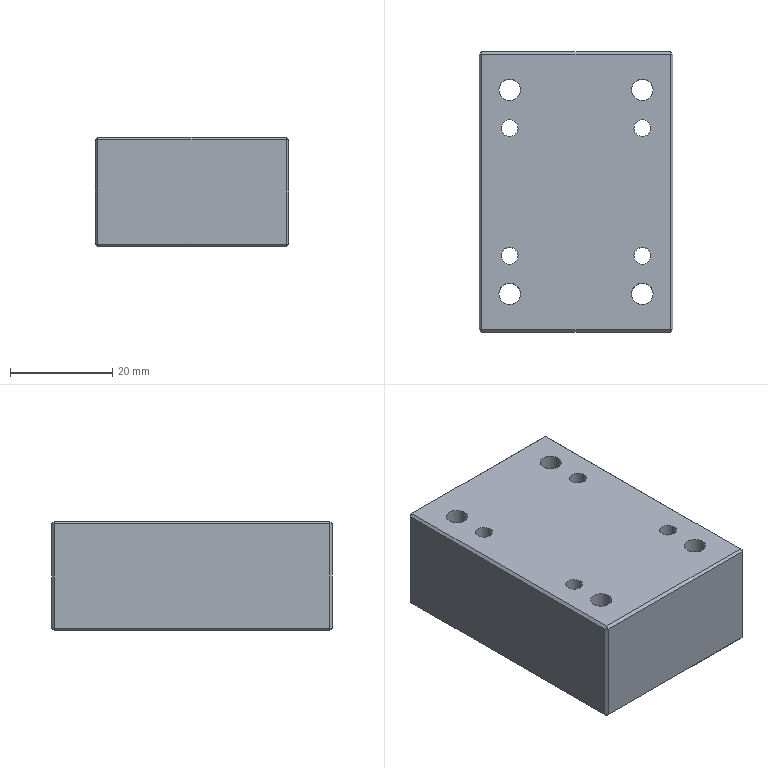Part | NX | 1 solid | 34 faces | box 38 x 55 x 21.5 mm | volume 42951 mm3 | plane 26 | cylinder 8 | commonest cylinder face diameters 3.3 x4 4.2 x4
STEP:
#1=CARTESIAN_POINT('',(-19.,-27.,0.5));
#2=VERTEX_POINT('',#1);
#3=CARTESIAN_POINT('',(-19.,-27.,21.));
#4=VERTEX_POINT('',#3);
#5=CARTESIAN_POINT('',(-19.,-27.,21.5));
#6=DIRECTION('',(0.,0.,1.));
#7=VECTOR('',#6,1000.);
#8=LINE('',#5,#7);
#9=EDGE_CURVE('',#2,#4,#8,.T.);
#10=ORIENTED_EDGE('',*,*,#9,.T.);
#11=CARTESIAN_POINT('',(-19.,27.,21.));
#12=VERTEX_POINT('',#11);
#13=CARTESIAN_POINT('',(-19.,27.5,21.));
#14=DIRECTION('',(0.,1.,0.));
#15=VECTOR('',#14,1000.);
#16=LINE('',#13,#15);
#17=EDGE_CURVE('',#4,#12,#16,.T.);
#18=ORIENTED_EDGE('',*,*,#17,.T.);
#19=CARTESIAN_POINT('',(-19.,27.,0.5));
#20=VERTEX_POINT('',#19);
#21=CARTESIAN_POINT('',(-19.,27.,21.5));
#22=DIRECTION('',(0.,0.,-1.));
#23=VECTOR('',#22,1000.);
#24=LINE('',#21,#23);
#25=EDGE_CURVE('',#12,#20,#24,.T.);
#26=ORIENTED_EDGE('',*,*,#25,.T.);
#27=CARTESIAN_POINT('',(-19.,-27.5,0.5));
#28=DIRECTION('',(0.,-1.,0.));
#29=VECTOR('',#28,1000.);
#30=LINE('',#27,#29);
#31=EDGE_CURVE('',#20,#2,#30,.T.);
#32=ORIENTED_EDGE('',*,*,#31,.T.);
#33=EDGE_LOOP('',(#10,#18,#26,#32));
#34=FACE_BOUND('',#33,.T.);
#35=CARTESIAN_POINT('',(-19.,27.5,21.5));
#36=DIRECTION('',(1.,0.,0.));
#37=DIRECTION('',(0.,1.,0.));
#38=AXIS2_PLACEMENT_3D('',#35,#36,#37);
#39=PLANE('',#38);
#40=ADVANCED_FACE('',(#34),#39,.F.);
#41=CARTESIAN_POINT('',(18.5,-27.5,21.));
#42=VERTEX_POINT('',#41);
#43=CARTESIAN_POINT('',(-18.5,-27.5,21.));
#44=VERTEX_POINT('',#43);
#45=CARTESIAN_POINT('',(19.,-27.5,21.));
#46=DIRECTION('',(-1.,0.,0.));
#47=VECTOR('',#46,1000.);
#48=LINE('',#45,#47);
#49=EDGE_CURVE('',#42,#44,#48,.T.);
#50=ORIENTED_EDGE('',*,*,#49,.T.);
#51=CARTESIAN_POINT('',(-18.5,-27.5,0.5));
#52=VERTEX_POINT('',#51);
#53=CARTESIAN_POINT('',(-18.5,-27.5,21.5));
#54=DIRECTION('',(0.,0.,-1.));
#55=VECTOR('',#54,1000.);
#56=LINE('',#53,#55);
#57=EDGE_CURVE('',#44,#52,#56,.T.);
#58=ORIENTED_EDGE('',*,*,#57,.T.);
#59=CARTESIAN_POINT('',(18.5,-27.5,0.5));
#60=VERTEX_POINT('',#59);
#61=CARTESIAN_POINT('',(19.,-27.5,0.5));
#62=DIRECTION('',(1.,0.,0.));
#63=VECTOR('',#62,1000.);
#64=LINE('',#61,#63);
#65=EDGE_CURVE('',#52,#60,#64,.T.);
#66=ORIENTED_EDGE('',*,*,#65,.T.);
#67=CARTESIAN_POINT('',(18.5,-27.5,21.5));
#68=DIRECTION('',(0.,0.,1.));
#69=VECTOR('',#68,1000.);
#70=LINE('',#67,#69);
#71=EDGE_CURVE('',#60,#42,#70,.T.);
#72=ORIENTED_EDGE('',*,*,#71,.T.);
#73=EDGE_LOOP('',(#50,#58,#66,#72));
#74=FACE_BOUND('',#73,.T.);
#75=CARTESIAN_POINT('',(19.,-27.5,21.5));
#76=DIRECTION('',(0.,1.,0.));
#77=DIRECTION('',(-1.,0.,0.));
#78=AXIS2_PLACEMENT_3D('',#75,#76,#77);
#79=PLANE('',#78);
#80=ADVANCED_FACE('',(#74),#79,.F.);
#81=CARTESIAN_POINT('',(19.,-27.,0.5));
#82=VERTEX_POINT('',#81);
#83=CARTESIAN_POINT('',(19.,27.,0.5));
#84=VERTEX_POINT('',#83);
#85=CARTESIAN_POINT('',(19.,27.5,0.5));
#86=DIRECTION('',(0.,1.,0.));
#87=VECTOR('',#86,1000.);
#88=LINE('',#85,#87);
#89=EDGE_CURVE('',#82,#84,#88,.T.);
#90=ORIENTED_EDGE('',*,*,#89,.T.);
#91=CARTESIAN_POINT('',(19.,27.,21.));
#92=VERTEX_POINT('',#91);
#93=CARTESIAN_POINT('',(19.,27.,21.5));
#94=DIRECTION('',(0.,0.,1.));
#95=VECTOR('',#94,1000.);
#96=LINE('',#93,#95);
#97=EDGE_CURVE('',#84,#92,#96,.T.);
#98=ORIENTED_EDGE('',*,*,#97,.T.);
#99=CARTESIAN_POINT('',(19.,-27.,21.));
#100=VERTEX_POINT('',#99);
#101=CARTESIAN_POINT('',(19.,27.5,21.));
#102=DIRECTION('',(0.,-1.,0.));
#103=VECTOR('',#102,1000.);
#104=LINE('',#101,#103);
#105=EDGE_CURVE('',#92,#100,#104,.T.);
#106=ORIENTED_EDGE('',*,*,#105,.T.);
#107=CARTESIAN_POINT('',(19.,-27.,21.5));
#108=DIRECTION('',(0.,0.,-1.));
#109=VECTOR('',#108,1000.);
#110=LINE('',#107,#109);
#111=EDGE_CURVE('',#100,#82,#110,.T.);
#112=ORIENTED_EDGE('',*,*,#111,.T.);
#113=EDGE_LOOP('',(#90,#98,#106,#112));
#114=FACE_BOUND('',#113,.T.);
#115=CARTESIAN_POINT('',(19.,27.5,21.5));
#116=DIRECTION('',(-1.,0.,0.));
#117=DIRECTION('',(0.,-1.,0.));
#118=AXIS2_PLACEMENT_3D('',#115,#116,#117);
#119=PLANE('',#118);
#120=ADVANCED_FACE('',(#114),#119,.F.);
#121=CARTESIAN_POINT('',(-18.5,27.5,21.));
#122=VERTEX_POINT('',#121);
#123=CARTESIAN_POINT('',(18.5,27.5,21.));
#124=VERTEX_POINT('',#123);
#125=CARTESIAN_POINT('',(19.,27.5,21.));
#126=DIRECTION('',(1.,0.,0.));
#127=VECTOR('',#126,1000.);
#128=LINE('',#125,#127);
#129=EDGE_CURVE('',#122,#124,#128,.T.);
#130=ORIENTED_EDGE('',*,*,#129,.T.);
#131=CARTESIAN_POINT('',(18.5,27.5,0.5));
#132=VERTEX_POINT('',#131);
#133=CARTESIAN_POINT('',(18.5,27.5,21.5));
#134=DIRECTION('',(0.,0.,-1.));
#135=VECTOR('',#134,1000.);
#136=LINE('',#133,#135);
#137=EDGE_CURVE('',#124,#132,#136,.T.);
#138=ORIENTED_EDGE('',*,*,#137,.T.);
#139=CARTESIAN_POINT('',(-18.5,27.5,0.5));
#140=VERTEX_POINT('',#139);
#141=CARTESIAN_POINT('',(-19.,27.5,0.5));
#142=DIRECTION('',(-1.,0.,0.));
#143=VECTOR('',#142,1000.);
#144=LINE('',#141,#143);
#145=EDGE_CURVE('',#132,#140,#144,.T.);
#146=ORIENTED_EDGE('',*,*,#145,.T.);
#147=CARTESIAN_POINT('',(-18.5,27.5,21.5));
#148=DIRECTION('',(0.,0.,1.));
#149=VECTOR('',#148,1000.);
#150=LINE('',#147,#149);
#151=EDGE_CURVE('',#140,#122,#150,.T.);
#152=ORIENTED_EDGE('',*,*,#151,.T.);
#153=EDGE_LOOP('',(#130,#138,#146,#152));
#154=FACE_BOUND('',#153,.T.);
#155=CARTESIAN_POINT('',(19.,27.5,21.5));
#156=DIRECTION('',(0.,-1.,0.));
#157=DIRECTION('',(1.,0.,0.));
#158=AXIS2_PLACEMENT_3D('',#155,#156,#157);
#159=PLANE('',#158);
#160=ADVANCED_FACE('',(#154),#159,.F.);
#161=CARTESIAN_POINT('',(18.5,-27.,21.5));
#162=VERTEX_POINT('',#161);
#163=CARTESIAN_POINT('',(18.5,27.,21.5));
#164=VERTEX_POINT('',#163);
#165=CARTESIAN_POINT('',(18.5,0.,21.5));
#166=DIRECTION('',(0.,1.,0.));
#167=VECTOR('',#166,1000.);
#168=LINE('',#165,#167);
#169=EDGE_CURVE('',#162,#164,#168,.T.);
#170=ORIENTED_EDGE('',*,*,#169,.T.);
#171=CARTESIAN_POINT('',(-18.5,27.,21.5));
#172=VERTEX_POINT('',#171);
#173=CARTESIAN_POINT('',(0.,27.,21.5));
#174=DIRECTION('',(-1.,0.,0.));
#175=VECTOR('',#174,1000.);
#176=LINE('',#173,#175);
#177=EDGE_CURVE('',#164,#172,#176,.T.);
#178=ORIENTED_EDGE('',*,*,#177,.T.);
#179=CARTESIAN_POINT('',(-18.5,-27.,21.5));
#180=VERTEX_POINT('',#179);
#181=CARTESIAN_POINT('',(-18.5,0.,21.5));
#182=DIRECTION('',(0.,-1.,0.));
#183=VECTOR('',#182,1000.);
#184=LINE('',#181,#183);
#185=EDGE_CURVE('',#172,#180,#184,.T.);
#186=ORIENTED_EDGE('',*,*,#185,.T.);
#187=CARTESIAN_POINT('',(0.,-27.,21.5));
#188=DIRECTION('',(1.,0.,0.));
#189=VECTOR('',#188,1000.);
#190=LINE('',#187,#189);
#191=EDGE_CURVE('',#180,#162,#190,.T.);
#192=ORIENTED_EDGE('',*,*,#191,.T.);
#193=EDGE_LOOP('',(#170,#178,#186,#192));
#194=FACE_BOUND('',#193,.T.);
#195=CARTESIAN_POINT('',(11.35,12.5,21.5));
#196=VERTEX_POINT('',#195);
#197=CARTESIAN_POINT('',(13.,12.5,21.5));
#198=DIRECTION('',(0.,0.,-1.));
#199=DIRECTION('',(-1.,0.,0.));
#200=AXIS2_PLACEMENT_3D('',#197,#198,#199);
#201=CIRCLE('',#200,1.65);
#202=EDGE_CURVE('',#196,#196,#201,.T.);
#203=ORIENTED_EDGE('',*,*,#202,.T.);
#204=EDGE_LOOP('',(#203));
#205=FACE_BOUND('',#204,.T.);
#206=CARTESIAN_POINT('',(-14.65,12.5,21.5));
#207=VERTEX_POINT('',#206);
#208=CARTESIAN_POINT('',(-13.,12.5,21.5));
#209=DIRECTION('',(0.,0.,-1.));
#210=DIRECTION('',(-1.,0.,0.));
#211=AXIS2_PLACEMENT_3D('',#208,#209,#210);
#212=CIRCLE('',#211,1.65);
#213=EDGE_CURVE('',#207,#207,#212,.T.);
#214=ORIENTED_EDGE('',*,*,#213,.T.);
#215=EDGE_LOOP('',(#214));
#216=FACE_BOUND('',#215,.T.);
#217=CARTESIAN_POINT('',(-14.65,-12.5,21.5));
#218=VERTEX_POINT('',#217);
#219=CARTESIAN_POINT('',(-13.,-12.5,21.5));
#220=DIRECTION('',(0.,0.,-1.));
#221=DIRECTION('',(-1.,0.,0.));
#222=AXIS2_PLACEMENT_3D('',#219,#220,#221);
#223=CIRCLE('',#222,1.65);
#224=EDGE_CURVE('',#218,#218,#223,.T.);
#225=ORIENTED_EDGE('',*,*,#224,.T.);
#226=EDGE_LOOP('',(#225));
#227=FACE_BOUND('',#226,.T.);
#228=CARTESIAN_POINT('',(11.35,-12.5,21.5));
#229=VERTEX_POINT('',#228);
#230=CARTESIAN_POINT('',(13.,-12.5,21.5));
#231=DIRECTION('',(0.,0.,-1.));
#232=DIRECTION('',(-1.,0.,0.));
#233=AXIS2_PLACEMENT_3D('',#230,#231,#232);
#234=CIRCLE('',#233,1.65);
#235=EDGE_CURVE('',#229,#229,#234,.T.);
#236=ORIENTED_EDGE('',*,*,#235,.T.);
#237=EDGE_LOOP('',(#236));
#238=FACE_BOUND('',#237,.T.);
#239=CARTESIAN_POINT('',(10.9,20.,21.5));
#240=VERTEX_POINT('',#239);
#241=CARTESIAN_POINT('',(13.,20.,21.5));
#242=DIRECTION('',(0.,0.,-1.));
#243=DIRECTION('',(-1.,0.,0.));
#244=AXIS2_PLACEMENT_3D('',#241,#242,#243);
#245=CIRCLE('',#244,2.1);
#246=EDGE_CURVE('',#240,#240,#245,.T.);
#247=ORIENTED_EDGE('',*,*,#246,.T.);
#248=EDGE_LOOP('',(#247));
#249=FACE_BOUND('',#248,.T.);
#250=CARTESIAN_POINT('',(10.9,-20.,21.5));
#251=VERTEX_POINT('',#250);
#252=CARTESIAN_POINT('',(13.,-20.,21.5));
#253=DIRECTION('',(0.,0.,-1.));
#254=DIRECTION('',(-1.,0.,0.));
#255=AXIS2_PLACEMENT_3D('',#252,#253,#254);
#256=CIRCLE('',#255,2.1);
#257=EDGE_CURVE('',#251,#251,#256,.T.);
#258=ORIENTED_EDGE('',*,*,#257,.T.);
#259=EDGE_LOOP('',(#258));
#260=FACE_BOUND('',#259,.T.);
#261=CARTESIAN_POINT('',(-15.1,-20.,21.5));
#262=VERTEX_POINT('',#261);
#263=CARTESIAN_POINT('',(-13.,-20.,21.5));
#264=DIRECTION('',(0.,0.,-1.));
#265=DIRECTION('',(-1.,0.,0.));
#266=AXIS2_PLACEMENT_3D('',#263,#264,#265);
#267=CIRCLE('',#266,2.1);
#268=EDGE_CURVE('',#262,#262,#267,.T.);
#269=ORIENTED_EDGE('',*,*,#268,.T.);
#270=EDGE_LOOP('',(#269));
#271=FACE_BOUND('',#270,.T.);
#272=CARTESIAN_POINT('',(-15.1,20.,21.5));
#273=VERTEX_POINT('',#272);
#274=CARTESIAN_POINT('',(-13.,20.,21.5));
#275=DIRECTION('',(0.,0.,-1.));
#276=DIRECTION('',(-1.,0.,0.));
#277=AXIS2_PLACEMENT_3D('',#274,#275,#276);
#278=CIRCLE('',#277,2.1);
#279=EDGE_CURVE('',#273,#273,#278,.T.);
#280=ORIENTED_EDGE('',*,*,#279,.T.);
#281=EDGE_LOOP('',(#280));
#282=FACE_BOUND('',#281,.T.);
#283=CARTESIAN_POINT('',(0.,0.,21.5));
#284=DIRECTION('',(0.,0.,-1.));
#285=DIRECTION('',(-1.,0.,0.));
#286=AXIS2_PLACEMENT_3D('',#283,#284,#285);
#287=PLANE('',#286);
#288=ADVANCED_FACE('',(#194,#205,#216,#227,#238,#249,#260,#271,#282),#287,.F.);
#289=CARTESIAN_POINT('',(-18.5,-27.,0.));
#290=VERTEX_POINT('',#289);
#291=CARTESIAN_POINT('',(-18.5,27.,0.));
#292=VERTEX_POINT('',#291);
#293=CARTESIAN_POINT('',(-18.5,27.5,0.));
#294=DIRECTION('',(0.,1.,0.));
#295=VECTOR('',#294,1000.);
#296=LINE('',#293,#295);
#297=EDGE_CURVE('',#290,#292,#296,.T.);
#298=ORIENTED_EDGE('',*,*,#297,.T.);
#299=CARTESIAN_POINT('',(18.5,27.,0.));
#300=VERTEX_POINT('',#299);
#301=CARTESIAN_POINT('',(19.,27.,0.));
#302=DIRECTION('',(1.,0.,0.));
#303=VECTOR('',#302,1000.);
#304=LINE('',#301,#303);
#305=EDGE_CURVE('',#292,#300,#304,.T.);
#306=ORIENTED_EDGE('',*,*,#305,.T.);
#307=CARTESIAN_POINT('',(18.5,-27.,0.));
#308=VERTEX_POINT('',#307);
#309=CARTESIAN_POINT('',(18.5,-27.5,0.));
#310=DIRECTION('',(0.,-1.,0.));
#311=VECTOR('',#310,1000.);
#312=LINE('',#309,#311);
#313=EDGE_CURVE('',#300,#308,#312,.T.);
#314=ORIENTED_EDGE('',*,*,#313,.T.);
#315=CARTESIAN_POINT('',(-19.,-27.,0.));
#316=DIRECTION('',(-1.,0.,0.));
#317=VECTOR('',#316,1000.);
#318=LINE('',#315,#317);
#319=EDGE_CURVE('',#308,#290,#318,.T.);
#320=ORIENTED_EDGE('',*,*,#319,.T.);
#321=EDGE_LOOP('',(#298,#306,#314,#320));
#322=FACE_BOUND('',#321,.T.);
#323=CARTESIAN_POINT('',(11.35,12.5,0.));
#324=VERTEX_POINT('',#323);
#325=CARTESIAN_POINT('',(13.,12.5,0.));
#326=DIRECTION('',(0.,0.,-1.));
#327=DIRECTION('',(-1.,0.,0.));
#328=AXIS2_PLACEMENT_3D('',#325,#326,#327);
#329=CIRCLE('',#328,1.65);
#330=EDGE_CURVE('',#324,#324,#329,.T.);
#331=ORIENTED_EDGE('',*,*,#330,.F.);
#332=EDGE_LOOP('',(#331));
#333=FACE_BOUND('',#332,.T.);
#334=CARTESIAN_POINT('',(-14.65,12.5,0.));
#335=VERTEX_POINT('',#334);
#336=CARTESIAN_POINT('',(-13.,12.5,0.));
#337=DIRECTION('',(0.,0.,-1.));
#338=DIRECTION('',(-1.,0.,0.));
#339=AXIS2_PLACEMENT_3D('',#336,#337,#338);
#340=CIRCLE('',#339,1.65);
#341=EDGE_CURVE('',#335,#335,#340,.T.);
#342=ORIENTED_EDGE('',*,*,#341,.F.);
#343=EDGE_LOOP('',(#342));
#344=FACE_BOUND('',#343,.T.);
#345=CARTESIAN_POINT('',(-14.65,-12.5,0.));
#346=VERTEX_POINT('',#345);
#347=CARTESIAN_POINT('',(-13.,-12.5,0.));
#348=DIRECTION('',(0.,0.,-1.));
#349=DIRECTION('',(-1.,0.,0.));
#350=AXIS2_PLACEMENT_3D('',#347,#348,#349);
#351=CIRCLE('',#350,1.65);
#352=EDGE_CURVE('',#346,#346,#351,.T.);
#353=ORIENTED_EDGE('',*,*,#352,.F.);
#354=EDGE_LOOP('',(#353));
#355=FACE_BOUND('',#354,.T.);
#356=CARTESIAN_POINT('',(11.35,-12.5,0.));
#357=VERTEX_POINT('',#356);
#358=CARTESIAN_POINT('',(13.,-12.5,0.));
#359=DIRECTION('',(0.,0.,-1.));
#360=DIRECTION('',(-1.,0.,0.));
#361=AXIS2_PLACEMENT_3D('',#358,#359,#360);
#362=CIRCLE('',#361,1.65);
#363=EDGE_CURVE('',#357,#357,#362,.T.);
#364=ORIENTED_EDGE('',*,*,#363,.F.);
#365=EDGE_LOOP('',(#364));
#366=FACE_BOUND('',#365,.T.);
#367=CARTESIAN_POINT('',(10.9,20.,0.));
#368=VERTEX_POINT('',#367);
#369=CARTESIAN_POINT('',(13.,20.,0.));
#370=DIRECTION('',(0.,0.,-1.));
#371=DIRECTION('',(-1.,0.,0.));
#372=AXIS2_PLACEMENT_3D('',#369,#370,#371);
#373=CIRCLE('',#372,2.1);
#374=EDGE_CURVE('',#368,#368,#373,.T.);
#375=ORIENTED_EDGE('',*,*,#374,.F.);
#376=EDGE_LOOP('',(#375));
#377=FACE_BOUND('',#376,.T.);
#378=CARTESIAN_POINT('',(10.9,-20.,0.));
#379=VERTEX_POINT('',#378);
#380=CARTESIAN_POINT('',(13.,-20.,0.));
#381=DIRECTION('',(0.,0.,-1.));
#382=DIRECTION('',(-1.,0.,0.));
#383=AXIS2_PLACEMENT_3D('',#380,#381,#382);
#384=CIRCLE('',#383,2.1);
#385=EDGE_CURVE('',#379,#379,#384,.T.);
#386=ORIENTED_EDGE('',*,*,#385,.F.);
#387=EDGE_LOOP('',(#386));
#388=FACE_BOUND('',#387,.T.);
#389=CARTESIAN_POINT('',(-15.1,-20.,0.));
#390=VERTEX_POINT('',#389);
#391=CARTESIAN_POINT('',(-13.,-20.,0.));
#392=DIRECTION('',(0.,0.,-1.));
#393=DIRECTION('',(-1.,0.,0.));
#394=AXIS2_PLACEMENT_3D('',#391,#392,#393);
#395=CIRCLE('',#394,2.1);
#396=EDGE_CURVE('',#390,#390,#395,.T.);
#397=ORIENTED_EDGE('',*,*,#396,.F.);
#398=EDGE_LOOP('',(#397));
#399=FACE_BOUND('',#398,.T.);
#400=CARTESIAN_POINT('',(-15.1,20.,0.));
#401=VERTEX_POINT('',#400);
#402=CARTESIAN_POINT('',(-13.,20.,0.));
#403=DIRECTION('',(0.,0.,-1.));
#404=DIRECTION('',(-1.,0.,0.));
#405=AXIS2_PLACEMENT_3D('',#402,#403,#404);
#406=CIRCLE('',#405,2.1);
#407=EDGE_CURVE('',#401,#401,#406,.T.);
#408=ORIENTED_EDGE('',*,*,#407,.F.);
#409=EDGE_LOOP('',(#408));
#410=FACE_BOUND('',#409,.T.);
#411=CARTESIAN_POINT('',(0.,0.,0.));
#412=DIRECTION('',(0.,0.,-1.));
#413=DIRECTION('',(-1.,0.,0.));
#414=AXIS2_PLACEMENT_3D('',#411,#412,#413);
#415=PLANE('',#414);
#416=ADVANCED_FACE('',(#322,#333,#344,#355,#366,#377,#388,#399,#410),#415,.T.);
#417=ORIENTED_EDGE('',*,*,#279,.F.);
#418=EDGE_LOOP('',(#417));
#419=FACE_BOUND('',#418,.T.);
#420=ORIENTED_EDGE('',*,*,#407,.T.);
#421=EDGE_LOOP('',(#420));
#422=FACE_BOUND('',#421,.T.);
#423=CARTESIAN_POINT('',(-13.,20.,0.));
#424=DIRECTION('',(0.,0.,-1.));
#425=DIRECTION('',(-1.,0.,0.));
#426=AXIS2_PLACEMENT_3D('',#423,#424,#425);
#427=CYLINDRICAL_SURFACE('',#426,2.1);
#428=ADVANCED_FACE('',(#419,#422),#427,.F.);
#429=ORIENTED_EDGE('',*,*,#268,.F.);
#430=EDGE_LOOP('',(#429));
#431=FACE_BOUND('',#430,.T.);
#432=ORIENTED_EDGE('',*,*,#396,.T.);
#433=EDGE_LOOP('',(#432));
#434=FACE_BOUND('',#433,.T.);
#435=CARTESIAN_POINT('',(-13.,-20.,0.));
#436=DIRECTION('',(0.,0.,-1.));
#437=DIRECTION('',(-1.,0.,0.));
#438=AXIS2_PLACEMENT_3D('',#435,#436,#437);
#439=CYLINDRICAL_SURFACE('',#438,2.1);
#440=ADVANCED_FACE('',(#431,#434),#439,.F.);
#441=ORIENTED_EDGE('',*,*,#257,.F.);
#442=EDGE_LOOP('',(#441));
#443=FACE_BOUND('',#442,.T.);
#444=ORIENTED_EDGE('',*,*,#385,.T.);
#445=EDGE_LOOP('',(#444));
#446=FACE_BOUND('',#445,.T.);
#447=CARTESIAN_POINT('',(13.,-20.,0.));
#448=DIRECTION('',(0.,0.,-1.));
#449=DIRECTION('',(-1.,0.,0.));
#450=AXIS2_PLACEMENT_3D('',#447,#448,#449);
#451=CYLINDRICAL_SURFACE('',#450,2.1);
#452=ADVANCED_FACE('',(#443,#446),#451,.F.);
#453=ORIENTED_EDGE('',*,*,#246,.F.);
#454=EDGE_LOOP('',(#453));
#455=FACE_BOUND('',#454,.T.);
#456=ORIENTED_EDGE('',*,*,#374,.T.);
#457=EDGE_LOOP('',(#456));
#458=FACE_BOUND('',#457,.T.);
#459=CARTESIAN_POINT('',(13.,20.,0.));
#460=DIRECTION('',(0.,0.,-1.));
#461=DIRECTION('',(-1.,0.,0.));
#462=AXIS2_PLACEMENT_3D('',#459,#460,#461);
#463=CYLINDRICAL_SURFACE('',#462,2.1);
#464=ADVANCED_FACE('',(#455,#458),#463,.F.);
#465=ORIENTED_EDGE('',*,*,#235,.F.);
#466=EDGE_LOOP('',(#465));
#467=FACE_BOUND('',#466,.T.);
#468=ORIENTED_EDGE('',*,*,#363,.T.);
#469=EDGE_LOOP('',(#468));
#470=FACE_BOUND('',#469,.T.);
#471=CARTESIAN_POINT('',(13.,-12.5,0.));
#472=DIRECTION('',(0.,0.,-1.));
#473=DIRECTION('',(-1.,0.,0.));
#474=AXIS2_PLACEMENT_3D('',#471,#472,#473);
#475=CYLINDRICAL_SURFACE('',#474,1.65);
#476=ADVANCED_FACE('',(#467,#470),#475,.F.);
#477=ORIENTED_EDGE('',*,*,#224,.F.);
#478=EDGE_LOOP('',(#477));
#479=FACE_BOUND('',#478,.T.);
#480=ORIENTED_EDGE('',*,*,#352,.T.);
#481=EDGE_LOOP('',(#480));
#482=FACE_BOUND('',#481,.T.);
#483=CARTESIAN_POINT('',(-13.,-12.5,0.));
#484=DIRECTION('',(0.,0.,-1.));
#485=DIRECTION('',(-1.,0.,0.));
#486=AXIS2_PLACEMENT_3D('',#483,#484,#485);
#487=CYLINDRICAL_SURFACE('',#486,1.65);
#488=ADVANCED_FACE('',(#479,#482),#487,.F.);
#489=ORIENTED_EDGE('',*,*,#213,.F.);
#490=EDGE_LOOP('',(#489));
#491=FACE_BOUND('',#490,.T.);
#492=ORIENTED_EDGE('',*,*,#341,.T.);
#493=EDGE_LOOP('',(#492));
#494=FACE_BOUND('',#493,.T.);
#495=CARTESIAN_POINT('',(-13.,12.5,0.));
#496=DIRECTION('',(0.,0.,-1.));
#497=DIRECTION('',(-1.,0.,0.));
#498=AXIS2_PLACEMENT_3D('',#495,#496,#497);
#499=CYLINDRICAL_SURFACE('',#498,1.65);
#500=ADVANCED_FACE('',(#491,#494),#499,.F.);
#501=ORIENTED_EDGE('',*,*,#202,.F.);
#502=EDGE_LOOP('',(#501));
#503=FACE_BOUND('',#502,.T.);
#504=ORIENTED_EDGE('',*,*,#330,.T.);
#505=EDGE_LOOP('',(#504));
#506=FACE_BOUND('',#505,.T.);
#507=CARTESIAN_POINT('',(13.,12.5,0.));
#508=DIRECTION('',(0.,0.,-1.));
#509=DIRECTION('',(-1.,0.,0.));
#510=AXIS2_PLACEMENT_3D('',#507,#508,#509);
#511=CYLINDRICAL_SURFACE('',#510,1.65);
#512=ADVANCED_FACE('',(#503,#506),#511,.F.);
#513=CARTESIAN_POINT('',(-19.,-27.,21.));
#514=DIRECTION('',(-0.7071,0.7071,0.));
#515=VECTOR('',#514,1000.);
#516=LINE('',#513,#515);
#517=EDGE_CURVE('',#4,#44,#516,.F.);
#518=ORIENTED_EDGE('',*,*,#517,.F.);
#519=ORIENTED_EDGE('',*,*,#9,.F.);
#520=CARTESIAN_POINT('',(-18.5,-27.5,0.5));
#521=DIRECTION('',(0.7071,-0.7071,0.));
#522=VECTOR('',#521,1000.);
#523=LINE('',#520,#522);
#524=EDGE_CURVE('',#52,#2,#523,.F.);
#525=ORIENTED_EDGE('',*,*,#524,.F.);
#526=ORIENTED_EDGE('',*,*,#57,.F.);
#527=EDGE_LOOP('',(#518,#519,#525,#526));
#528=FACE_BOUND('',#527,.T.);
#529=CARTESIAN_POINT('',(-18.5,-27.5,21.5));
#530=DIRECTION('',(0.7071,0.7071,0.));
#531=DIRECTION('',(0.,0.,-1.));
#532=AXIS2_PLACEMENT_3D('',#529,#530,#531);
#533=PLANE('',#532);
#534=ADVANCED_FACE('',(#528),#533,.F.);
#535=CARTESIAN_POINT('',(-19.,-27.,21.));
#536=DIRECTION('',(0.7071,0.,0.7071));
#537=VECTOR('',#536,1000.);
#538=LINE('',#535,#537);
#539=EDGE_CURVE('',#4,#180,#538,.T.);
#540=ORIENTED_EDGE('',*,*,#539,.F.);
#541=ORIENTED_EDGE('',*,*,#517,.T.);
#542=CARTESIAN_POINT('',(-18.5,-27.25,21.25));
#543=DIRECTION('',(0.,-0.7071,-0.7071));
#544=VECTOR('',#543,1000.);
#545=LINE('',#542,#544);
#546=EDGE_CURVE('',#180,#44,#545,.T.);
#547=ORIENTED_EDGE('',*,*,#546,.F.);
#548=EDGE_LOOP('',(#540,#541,#547));
#549=FACE_BOUND('',#548,.T.);
#550=CARTESIAN_POINT('',(-19.,-27.,21.));
#551=DIRECTION('',(-0.5774,-0.5774,0.5774));
#552=DIRECTION('',(0.,-0.7071,-0.7071));
#553=AXIS2_PLACEMENT_3D('',#550,#551,#552);
#554=PLANE('',#553);
#555=ADVANCED_FACE('',(#549),#554,.T.);
#556=CARTESIAN_POINT('',(-18.5,-27.5,0.5));
#557=DIRECTION('',(0.,-0.7071,0.7071));
#558=VECTOR('',#557,1000.);
#559=LINE('',#556,#558);
#560=EDGE_CURVE('',#52,#290,#559,.F.);
#561=ORIENTED_EDGE('',*,*,#560,.F.);
#562=ORIENTED_EDGE('',*,*,#524,.T.);
#563=CARTESIAN_POINT('',(-18.75,-27.,0.25));
#564=DIRECTION('',(0.7071,0.,-0.7071));
#565=VECTOR('',#564,1000.);
#566=LINE('',#563,#565);
#567=EDGE_CURVE('',#290,#2,#566,.F.);
#568=ORIENTED_EDGE('',*,*,#567,.F.);
#569=EDGE_LOOP('',(#561,#562,#568));
#570=FACE_BOUND('',#569,.T.);
#571=CARTESIAN_POINT('',(-18.5,-27.5,0.5));
#572=DIRECTION('',(-0.5774,-0.5774,-0.5774));
#573=DIRECTION('',(0.,0.7071,-0.7071));
#574=AXIS2_PLACEMENT_3D('',#571,#572,#573);
#575=PLANE('',#574);
#576=ADVANCED_FACE('',(#570),#575,.T.);
#577=ORIENTED_EDGE('',*,*,#546,.T.);
#578=ORIENTED_EDGE('',*,*,#49,.F.);
#579=CARTESIAN_POINT('',(18.5,-27.,21.5));
#580=DIRECTION('',(0.,0.7071,0.7071));
#581=VECTOR('',#580,1000.);
#582=LINE('',#579,#581);
#583=EDGE_CURVE('',#162,#42,#582,.F.);
#584=ORIENTED_EDGE('',*,*,#583,.F.);
#585=ORIENTED_EDGE('',*,*,#191,.F.);
#586=EDGE_LOOP('',(#577,#578,#584,#585));
#587=FACE_BOUND('',#586,.T.);
#588=CARTESIAN_POINT('',(0.,-27.,21.5));
#589=DIRECTION('',(0.,0.7071,-0.7071));
#590=DIRECTION('',(1.,0.,0.));
#591=AXIS2_PLACEMENT_3D('',#588,#589,#590);
#592=PLANE('',#591);
#593=ADVANCED_FACE('',(#587),#592,.F.);
#594=ORIENTED_EDGE('',*,*,#539,.T.);
#595=ORIENTED_EDGE('',*,*,#185,.F.);
#596=CARTESIAN_POINT('',(-18.5,27.,21.5));
#597=DIRECTION('',(-0.7071,0.,-0.7071));
#598=VECTOR('',#597,1000.);
#599=LINE('',#596,#598);
#600=EDGE_CURVE('',#12,#172,#599,.F.);
#601=ORIENTED_EDGE('',*,*,#600,.F.);
#602=ORIENTED_EDGE('',*,*,#17,.F.);
#603=EDGE_LOOP('',(#594,#595,#601,#602));
#604=FACE_BOUND('',#603,.T.);
#605=CARTESIAN_POINT('',(-18.5,0.,21.5));
#606=DIRECTION('',(0.7071,0.,-0.7071));
#607=DIRECTION('',(0.,-1.,0.));
#608=AXIS2_PLACEMENT_3D('',#605,#606,#607);
#609=PLANE('',#608);
#610=ADVANCED_FACE('',(#604),#609,.F.);
#611=CARTESIAN_POINT('',(-19.,27.,0.5));
#612=DIRECTION('',(-0.7071,-0.7071,0.));
#613=VECTOR('',#612,1000.);
#614=LINE('',#611,#613);
#615=EDGE_CURVE('',#20,#140,#614,.F.);
#616=ORIENTED_EDGE('',*,*,#615,.F.);
#617=ORIENTED_EDGE('',*,*,#25,.F.);
#618=CARTESIAN_POINT('',(-18.75,27.25,21.));
#619=DIRECTION('',(0.7071,0.7071,0.));
#620=VECTOR('',#619,1000.);
#621=LINE('',#618,#620);
#622=EDGE_CURVE('',#122,#12,#621,.F.);
#623=ORIENTED_EDGE('',*,*,#622,.F.);
#624=ORIENTED_EDGE('',*,*,#151,.F.);
#625=EDGE_LOOP('',(#616,#617,#623,#624));
#626=FACE_BOUND('',#625,.T.);
#627=CARTESIAN_POINT('',(-19.,27.,21.5));
#628=DIRECTION('',(0.7071,-0.7071,0.));
#629=DIRECTION('',(0.,0.,-1.));
#630=AXIS2_PLACEMENT_3D('',#627,#628,#629);
#631=PLANE('',#630);
#632=ADVANCED_FACE('',(#626),#631,.F.);
#633=ORIENTED_EDGE('',*,*,#567,.T.);
#634=ORIENTED_EDGE('',*,*,#31,.F.);
#635=CARTESIAN_POINT('',(-19.,27.,0.5));
#636=DIRECTION('',(-0.7071,0.,0.7071));
#637=VECTOR('',#636,1000.);
#638=LINE('',#635,#637);
#639=EDGE_CURVE('',#292,#20,#638,.T.);
#640=ORIENTED_EDGE('',*,*,#639,.F.);
#641=ORIENTED_EDGE('',*,*,#297,.F.);
#642=EDGE_LOOP('',(#633,#634,#640,#641));
#643=FACE_BOUND('',#642,.T.);
#644=CARTESIAN_POINT('',(-19.,27.5,0.5));
#645=DIRECTION('',(-0.7071,0.,-0.7071));
#646=DIRECTION('',(0.,1.,0.));
#647=AXIS2_PLACEMENT_3D('',#644,#645,#646);
#648=PLANE('',#647);
#649=ADVANCED_FACE('',(#643),#648,.T.);
#650=ORIENTED_EDGE('',*,*,#560,.T.);
#651=ORIENTED_EDGE('',*,*,#319,.F.);
#652=CARTESIAN_POINT('',(18.5,-27.25,0.25));
#653=DIRECTION('',(0.,0.7071,-0.7071));
#654=VECTOR('',#653,1000.);
#655=LINE('',#652,#654);
#656=EDGE_CURVE('',#60,#308,#655,.T.);
#657=ORIENTED_EDGE('',*,*,#656,.F.);
#658=ORIENTED_EDGE('',*,*,#65,.F.);
#659=EDGE_LOOP('',(#650,#651,#657,#658));
#660=FACE_BOUND('',#659,.T.);
#661=CARTESIAN_POINT('',(19.,-27.5,0.5));
#662=DIRECTION('',(0.,-0.7071,-0.7071));
#663=DIRECTION('',(-1.,0.,0.));
#664=AXIS2_PLACEMENT_3D('',#661,#662,#663);
#665=PLANE('',#664);
#666=ADVANCED_FACE('',(#660),#665,.T.);
#667=CARTESIAN_POINT('',(18.75,-27.25,21.));
#668=DIRECTION('',(-0.7071,-0.7071,0.));
#669=VECTOR('',#668,1000.);
#670=LINE('',#667,#669);
#671=EDGE_CURVE('',#42,#100,#670,.F.);
#672=ORIENTED_EDGE('',*,*,#671,.F.);
#673=ORIENTED_EDGE('',*,*,#71,.F.);
#674=CARTESIAN_POINT('',(19.,-27.,0.5));
#675=DIRECTION('',(0.7071,0.7071,0.));
#676=VECTOR('',#675,1000.);
#677=LINE('',#674,#676);
#678=EDGE_CURVE('',#82,#60,#677,.F.);
#679=ORIENTED_EDGE('',*,*,#678,.F.);
#680=ORIENTED_EDGE('',*,*,#111,.F.);
#681=EDGE_LOOP('',(#672,#673,#679,#680));
#682=FACE_BOUND('',#681,.T.);
#683=CARTESIAN_POINT('',(19.,-27.,21.5));
#684=DIRECTION('',(-0.7071,0.7071,0.));
#685=DIRECTION('',(0.,0.,-1.));
#686=AXIS2_PLACEMENT_3D('',#683,#684,#685);
#687=PLANE('',#686);
#688=ADVANCED_FACE('',(#682),#687,.F.);
#689=ORIENTED_EDGE('',*,*,#583,.T.);
#690=ORIENTED_EDGE('',*,*,#671,.T.);
#691=CARTESIAN_POINT('',(18.5,-27.,21.5));
#692=DIRECTION('',(0.7071,0.,-0.7071));
#693=VECTOR('',#692,1000.);
#694=LINE('',#691,#693);
#695=EDGE_CURVE('',#162,#100,#694,.T.);
#696=ORIENTED_EDGE('',*,*,#695,.F.);
#697=EDGE_LOOP('',(#689,#690,#696));
#698=FACE_BOUND('',#697,.T.);
#699=CARTESIAN_POINT('',(18.5,-27.,21.5));
#700=DIRECTION('',(0.5774,-0.5774,0.5774));
#701=DIRECTION('',(0.7071,0.7071,0.));
#702=AXIS2_PLACEMENT_3D('',#699,#700,#701);
#703=PLANE('',#702);
#704=ADVANCED_FACE('',(#698),#703,.T.);
#705=ORIENTED_EDGE('',*,*,#622,.T.);
#706=ORIENTED_EDGE('',*,*,#600,.T.);
#707=CARTESIAN_POINT('',(-18.5,27.,21.5));
#708=DIRECTION('',(0.,-0.7071,0.7071));
#709=VECTOR('',#708,1000.);
#710=LINE('',#707,#709);
#711=EDGE_CURVE('',#122,#172,#710,.T.);
#712=ORIENTED_EDGE('',*,*,#711,.F.);
#713=EDGE_LOOP('',(#705,#706,#712));
#714=FACE_BOUND('',#713,.T.);
#715=CARTESIAN_POINT('',(-18.5,27.,21.5));
#716=DIRECTION('',(-0.5774,0.5774,0.5774));
#717=DIRECTION('',(0.,-0.7071,0.7071));
#718=AXIS2_PLACEMENT_3D('',#715,#716,#717);
#719=PLANE('',#718);
#720=ADVANCED_FACE('',(#714),#719,.T.);
#721=ORIENTED_EDGE('',*,*,#639,.T.);
#722=ORIENTED_EDGE('',*,*,#615,.T.);
#723=CARTESIAN_POINT('',(-18.5,27.25,0.25));
#724=DIRECTION('',(0.,-0.7071,-0.7071));
#725=VECTOR('',#724,1000.);
#726=LINE('',#723,#725);
#727=EDGE_CURVE('',#292,#140,#726,.F.);
#728=ORIENTED_EDGE('',*,*,#727,.F.);
#729=EDGE_LOOP('',(#721,#722,#728));
#730=FACE_BOUND('',#729,.T.);
#731=CARTESIAN_POINT('',(-19.,27.,0.5));
#732=DIRECTION('',(-0.5774,0.5774,-0.5774));
#733=DIRECTION('',(0.,0.7071,0.7071));
#734=AXIS2_PLACEMENT_3D('',#731,#732,#733);
#735=PLANE('',#734);
#736=ADVANCED_FACE('',(#730),#735,.T.);
#737=ORIENTED_EDGE('',*,*,#678,.T.);
#738=ORIENTED_EDGE('',*,*,#656,.T.);
#739=CARTESIAN_POINT('',(19.,-27.,0.5));
#740=DIRECTION('',(0.7071,0.,0.7071));
#741=VECTOR('',#740,1000.);
#742=LINE('',#739,#741);
#743=EDGE_CURVE('',#82,#308,#742,.F.);
#744=ORIENTED_EDGE('',*,*,#743,.F.);
#745=EDGE_LOOP('',(#737,#738,#744));
#746=FACE_BOUND('',#745,.T.);
#747=CARTESIAN_POINT('',(19.,-27.,0.5));
#748=DIRECTION('',(0.5774,-0.5774,-0.5774));
#749=DIRECTION('',(0.,0.7071,-0.7071));
#750=AXIS2_PLACEMENT_3D('',#747,#748,#749);
#751=PLANE('',#750);
#752=ADVANCED_FACE('',(#746),#751,.T.);
#753=ORIENTED_EDGE('',*,*,#695,.T.);
#754=ORIENTED_EDGE('',*,*,#105,.F.);
#755=CARTESIAN_POINT('',(19.,27.,21.));
#756=DIRECTION('',(-0.7071,0.,0.7071));
#757=VECTOR('',#756,1000.);
#758=LINE('',#755,#757);
#759=EDGE_CURVE('',#164,#92,#758,.F.);
#760=ORIENTED_EDGE('',*,*,#759,.F.);
#761=ORIENTED_EDGE('',*,*,#169,.F.);
#762=EDGE_LOOP('',(#753,#754,#760,#761));
#763=FACE_BOUND('',#762,.T.);
#764=CARTESIAN_POINT('',(18.5,0.,21.5));
#765=DIRECTION('',(-0.7071,0.,-0.7071));
#766=DIRECTION('',(0.,1.,0.));
#767=AXIS2_PLACEMENT_3D('',#764,#765,#766);
#768=PLANE('',#767);
#769=ADVANCED_FACE('',(#763),#768,.F.);
#770=ORIENTED_EDGE('',*,*,#711,.T.);
#771=ORIENTED_EDGE('',*,*,#177,.F.);
#772=CARTESIAN_POINT('',(18.5,27.25,21.25));
#773=DIRECTION('',(0.,0.7071,-0.7071));
#774=VECTOR('',#773,1000.);
#775=LINE('',#772,#774);
#776=EDGE_CURVE('',#124,#164,#775,.F.);
#777=ORIENTED_EDGE('',*,*,#776,.F.);
#778=ORIENTED_EDGE('',*,*,#129,.F.);
#779=EDGE_LOOP('',(#770,#771,#777,#778));
#780=FACE_BOUND('',#779,.T.);
#781=CARTESIAN_POINT('',(0.,27.,21.5));
#782=DIRECTION('',(0.,-0.7071,-0.7071));
#783=DIRECTION('',(-1.,0.,0.));
#784=AXIS2_PLACEMENT_3D('',#781,#782,#783);
#785=PLANE('',#784);
#786=ADVANCED_FACE('',(#780),#785,.F.);
#787=ORIENTED_EDGE('',*,*,#727,.T.);
#788=ORIENTED_EDGE('',*,*,#145,.F.);
#789=CARTESIAN_POINT('',(18.5,27.5,0.5));
#790=DIRECTION('',(0.,0.7071,0.7071));
#791=VECTOR('',#790,1000.);
#792=LINE('',#789,#791);
#793=EDGE_CURVE('',#300,#132,#792,.T.);
#794=ORIENTED_EDGE('',*,*,#793,.F.);
#795=ORIENTED_EDGE('',*,*,#305,.F.);
#796=EDGE_LOOP('',(#787,#788,#794,#795));
#797=FACE_BOUND('',#796,.T.);
#798=CARTESIAN_POINT('',(19.,27.5,0.5));
#799=DIRECTION('',(0.,0.7071,-0.7071));
#800=DIRECTION('',(1.,0.,0.));
#801=AXIS2_PLACEMENT_3D('',#798,#799,#800);
#802=PLANE('',#801);
#803=ADVANCED_FACE('',(#797),#802,.T.);
#804=ORIENTED_EDGE('',*,*,#743,.T.);
#805=ORIENTED_EDGE('',*,*,#313,.F.);
#806=CARTESIAN_POINT('',(18.75,27.,0.25));
#807=DIRECTION('',(-0.7071,0.,-0.7071));
#808=VECTOR('',#807,1000.);
#809=LINE('',#806,#808);
#810=EDGE_CURVE('',#84,#300,#809,.T.);
#811=ORIENTED_EDGE('',*,*,#810,.F.);
#812=ORIENTED_EDGE('',*,*,#89,.F.);
#813=EDGE_LOOP('',(#804,#805,#811,#812));
#814=FACE_BOUND('',#813,.T.);
#815=CARTESIAN_POINT('',(19.,27.5,0.5));
#816=DIRECTION('',(0.7071,0.,-0.7071));
#817=DIRECTION('',(0.,-1.,0.));
#818=AXIS2_PLACEMENT_3D('',#815,#816,#817);
#819=PLANE('',#818);
#820=ADVANCED_FACE('',(#814),#819,.T.);
#821=ORIENTED_EDGE('',*,*,#776,.T.);
#822=ORIENTED_EDGE('',*,*,#759,.T.);
#823=CARTESIAN_POINT('',(19.,27.,21.));
#824=DIRECTION('',(0.7071,-0.7071,0.));
#825=VECTOR('',#824,1000.);
#826=LINE('',#823,#825);
#827=EDGE_CURVE('',#124,#92,#826,.T.);
#828=ORIENTED_EDGE('',*,*,#827,.F.);
#829=EDGE_LOOP('',(#821,#822,#828));
#830=FACE_BOUND('',#829,.T.);
#831=CARTESIAN_POINT('',(19.,27.,21.));
#832=DIRECTION('',(0.5774,0.5774,0.5774));
#833=DIRECTION('',(-0.7071,0.7071,0.));
#834=AXIS2_PLACEMENT_3D('',#831,#832,#833);
#835=PLANE('',#834);
#836=ADVANCED_FACE('',(#830),#835,.T.);
#837=ORIENTED_EDGE('',*,*,#810,.T.);
#838=ORIENTED_EDGE('',*,*,#793,.T.);
#839=CARTESIAN_POINT('',(18.5,27.5,0.5));
#840=DIRECTION('',(-0.7071,0.7071,0.));
#841=VECTOR('',#840,1000.);
#842=LINE('',#839,#841);
#843=EDGE_CURVE('',#84,#132,#842,.T.);
#844=ORIENTED_EDGE('',*,*,#843,.F.);
#845=EDGE_LOOP('',(#837,#838,#844));
#846=FACE_BOUND('',#845,.T.);
#847=CARTESIAN_POINT('',(18.5,27.5,0.5));
#848=DIRECTION('',(0.5774,0.5774,-0.5774));
#849=DIRECTION('',(-0.7071,0.,-0.7071));
#850=AXIS2_PLACEMENT_3D('',#847,#848,#849);
#851=PLANE('',#850);
#852=ADVANCED_FACE('',(#846),#851,.T.);
#853=ORIENTED_EDGE('',*,*,#827,.T.);
#854=ORIENTED_EDGE('',*,*,#97,.F.);
#855=ORIENTED_EDGE('',*,*,#843,.T.);
#856=ORIENTED_EDGE('',*,*,#137,.F.);
#857=EDGE_LOOP('',(#853,#854,#855,#856));
#858=FACE_BOUND('',#857,.T.);
#859=CARTESIAN_POINT('',(18.5,27.5,21.5));
#860=DIRECTION('',(-0.7071,-0.7071,0.));
#861=DIRECTION('',(0.,0.,-1.));
#862=AXIS2_PLACEMENT_3D('',#859,#860,#861);
#863=PLANE('',#862);
#864=ADVANCED_FACE('',(#858),#863,.F.);
#865=CLOSED_SHELL('',(#40,#80,#120,#160,#288,#416,#428,#440,#452,#464,#476,#488,#500,#512,#534,#555,#576,#593,#610,#632,#649,#666,#688,#704,#720,#736,#752,#769,#786,#803,#820,#836,#852,#864));
#866=MANIFOLD_SOLID_BREP('',#865);
#867=(LENGTH_UNIT()NAMED_UNIT(*)SI_UNIT(.MILLI.,.METRE.));
#868=UNCERTAINTY_MEASURE_WITH_UNIT(LENGTH_MEASURE(0.00001),#867,'','');
#869=(NAMED_UNIT(*)PLANE_ANGLE_UNIT()SI_UNIT($,.RADIAN.));
#870=(NAMED_UNIT(*)SI_UNIT($,.STERADIAN.)SOLID_ANGLE_UNIT());
#871=(GEOMETRIC_REPRESENTATION_CONTEXT(3)GLOBAL_UNCERTAINTY_ASSIGNED_CONTEXT((#868))GLOBAL_UNIT_ASSIGNED_CONTEXT((#867,#869,#870))REPRESENTATION_CONTEXT('',''));
#872=ADVANCED_BREP_SHAPE_REPRESENTATION('',(#866),#871);